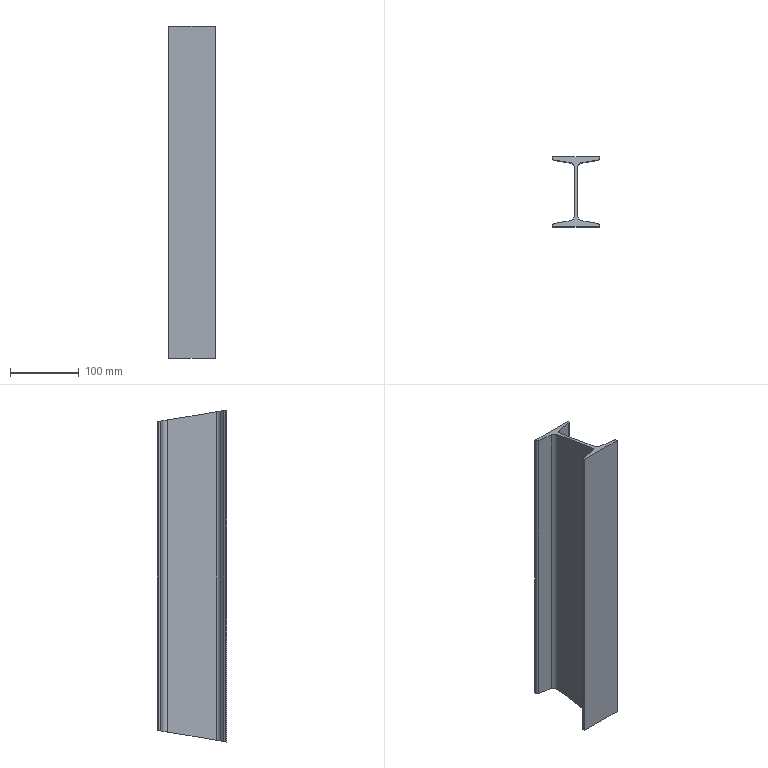Part | SolidWorks | features BaseBody 1 | 1 solid | 22 faces | box 67.6 x 101.6 x 482.765 mm | volume 647373 mm3 | plane 14 | cylinder 8 | commonest cylinder face diameters 5.6 x4 14.8 x4
STEP:
#1=CARTESIAN_POINT('',(-9.126,-3.883,0.));
#2=VERTEX_POINT('',#1);
#3=CARTESIAN_POINT('',(58.474,-3.883,0.));
#4=VERTEX_POINT('',#3);
#5=CARTESIAN_POINT('',(58.474,-3.883,0.));
#6=DIRECTION('',(1.,0.,0.));
#7=VECTOR('',#6,1000.);
#8=LINE('',#5,#7);
#9=EDGE_CURVE('',#2,#4,#8,.T.);
#10=ORIENTED_EDGE('',*,*,#9,.T.);
#11=CARTESIAN_POINT('',(58.474,-3.883,482.765));
#12=VERTEX_POINT('',#11);
#13=CARTESIAN_POINT('',(58.474,-3.883,0.));
#14=DIRECTION('',(0.,0.,1.));
#15=VECTOR('',#14,1000.);
#16=LINE('',#13,#15);
#17=EDGE_CURVE('',#4,#12,#16,.T.);
#18=ORIENTED_EDGE('',*,*,#17,.T.);
#19=CARTESIAN_POINT('',(-9.126,-3.883,482.765));
#20=VERTEX_POINT('',#19);
#21=CARTESIAN_POINT('',(58.474,-3.883,482.765));
#22=DIRECTION('',(-1.,0.,0.));
#23=VECTOR('',#22,1000.);
#24=LINE('',#21,#23);
#25=EDGE_CURVE('',#12,#20,#24,.T.);
#26=ORIENTED_EDGE('',*,*,#25,.T.);
#27=CARTESIAN_POINT('',(-9.126,-3.883,0.));
#28=DIRECTION('',(0.,0.,-1.));
#29=VECTOR('',#28,1000.);
#30=LINE('',#27,#29);
#31=EDGE_CURVE('',#20,#2,#30,.T.);
#32=ORIENTED_EDGE('',*,*,#31,.T.);
#33=EDGE_LOOP('',(#10,#18,#26,#32));
#34=FACE_OUTER_BOUND('',#33,.T.);
#35=CARTESIAN_POINT('',(58.474,-3.883,0.));
#36=DIRECTION('',(0.,-1.,0.));
#37=DIRECTION('',(0.,0.,-1.));
#38=AXIS2_PLACEMENT_3D('',#35,#36,#37);
#39=PLANE('',#38);
#40=ADVANCED_FACE('',(#34),#39,.T.);
#41=CARTESIAN_POINT('',(58.474,-1.913,482.435));
#42=VERTEX_POINT('',#41);
#43=CARTESIAN_POINT('',(58.474,-1.913,482.435));
#44=DIRECTION('',(0.,-0.9863,0.165));
#45=VECTOR('',#44,1000.);
#46=LINE('',#43,#45);
#47=EDGE_CURVE('',#42,#12,#46,.T.);
#48=ORIENTED_EDGE('',*,*,#47,.T.);
#49=ORIENTED_EDGE('',*,*,#17,.F.);
#50=CARTESIAN_POINT('',(58.474,-1.913,0.3297));
#51=VERTEX_POINT('',#50);
#52=CARTESIAN_POINT('',(58.474,-3.883,0.));
#53=DIRECTION('',(0.,0.9863,0.165));
#54=VECTOR('',#53,1000.);
#55=LINE('',#52,#54);
#56=EDGE_CURVE('',#4,#51,#55,.T.);
#57=ORIENTED_EDGE('',*,*,#56,.T.);
#58=CARTESIAN_POINT('',(58.474,-1.913,0.));
#59=DIRECTION('',(0.,0.,1.));
#60=VECTOR('',#59,1000.);
#61=LINE('',#58,#60);
#62=EDGE_CURVE('',#51,#42,#61,.T.);
#63=ORIENTED_EDGE('',*,*,#62,.T.);
#64=EDGE_LOOP('',(#48,#49,#57,#63));
#65=FACE_OUTER_BOUND('',#64,.T.);
#66=CARTESIAN_POINT('',(58.474,-1.913,0.));
#67=DIRECTION('',(1.,0.,0.));
#68=DIRECTION('',(0.,0.,-1.));
#69=AXIS2_PLACEMENT_3D('',#66,#67,#68);
#70=PLANE('',#69);
#71=ADVANCED_FACE('',(#65),#70,.T.);
#72=CARTESIAN_POINT('',(33.252,4.678,1.433));
#73=VERTEX_POINT('',#72);
#74=CARTESIAN_POINT('',(56.136,0.8486,0.7919));
#75=VERTEX_POINT('',#74);
#76=CARTESIAN_POINT('',(33.252,4.678,1.433));
#77=DIRECTION('',(0.9859,-0.165,-0.02761));
#78=VECTOR('',#77,1000.);
#79=LINE('',#76,#78);
#80=EDGE_CURVE('',#73,#75,#79,.T.);
#81=ORIENTED_EDGE('',*,*,#80,.T.);
#82=CARTESIAN_POINT('',(56.136,0.8486,0.7919));
#83=CARTESIAN_POINT('',(57.548,0.6122,0.7523));
#84=CARTESIAN_POINT('',(58.474,-0.4808,0.5694));
#85=CARTESIAN_POINT('',(58.474,-1.913,0.3297));
#86=(BOUNDED_CURVE()B_SPLINE_CURVE(3,(#82,#83,#84,#85),.UNSPECIFIED.,.F.,.F.)B_SPLINE_CURVE_WITH_KNOTS((4,4),(0.1658,1.571),.UNSPECIFIED.)CURVE()GEOMETRIC_REPRESENTATION_ITEM()RATIONAL_B_SPLINE_CURVE((1.,0.8422,0.8422,1.))REPRESENTATION_ITEM(''));
#87=EDGE_CURVE('',#75,#51,#86,.T.);
#88=ORIENTED_EDGE('',*,*,#87,.T.);
#89=ORIENTED_EDGE('',*,*,#56,.F.);
#90=ORIENTED_EDGE('',*,*,#9,.F.);
#91=CARTESIAN_POINT('',(-9.126,-1.913,0.3297));
#92=VERTEX_POINT('',#91);
#93=CARTESIAN_POINT('',(-9.126,46.917,8.501));
#94=DIRECTION('',(0.,0.9863,0.165));
#95=VECTOR('',#94,1000.);
#96=LINE('',#93,#95);
#97=EDGE_CURVE('',#2,#92,#96,.T.);
#98=ORIENTED_EDGE('',*,*,#97,.T.);
#99=CARTESIAN_POINT('',(-6.788,0.8486,0.7919));
#100=VERTEX_POINT('',#99);
#101=CARTESIAN_POINT('',(-9.126,-1.913,0.3297));
#102=CARTESIAN_POINT('',(-9.126,-0.4808,0.5694));
#103=CARTESIAN_POINT('',(-8.201,0.6122,0.7523));
#104=CARTESIAN_POINT('',(-6.788,0.8486,0.7919));
#105=(BOUNDED_CURVE()B_SPLINE_CURVE(3,(#101,#102,#103,#104),.UNSPECIFIED.,.F.,.T.)B_SPLINE_CURVE_WITH_KNOTS((4,4),(4.712,6.117),.UNSPECIFIED.)CURVE()GEOMETRIC_REPRESENTATION_ITEM()RATIONAL_B_SPLINE_CURVE((1.,0.8422,0.8422,1.))REPRESENTATION_ITEM(''));
#106=EDGE_CURVE('',#92,#100,#105,.T.);
#107=ORIENTED_EDGE('',*,*,#106,.T.);
#108=CARTESIAN_POINT('',(16.095,4.678,1.433));
#109=VERTEX_POINT('',#108);
#110=CARTESIAN_POINT('',(-6.788,0.8486,0.7919));
#111=DIRECTION('',(0.9859,0.165,0.02761));
#112=VECTOR('',#111,1000.);
#113=LINE('',#110,#112);
#114=EDGE_CURVE('',#100,#109,#113,.T.);
#115=ORIENTED_EDGE('',*,*,#114,.T.);
#116=CARTESIAN_POINT('',(22.274,11.977,2.654));
#117=VERTEX_POINT('',#116);
#118=CARTESIAN_POINT('',(16.095,4.678,1.433));
#119=CARTESIAN_POINT('',(19.828,5.303,1.537));
#120=CARTESIAN_POINT('',(22.274,8.192,2.021));
#121=CARTESIAN_POINT('',(22.274,11.977,2.654));
#122=(BOUNDED_CURVE()B_SPLINE_CURVE(3,(#118,#119,#120,#121),.UNSPECIFIED.,.F.,.F.)B_SPLINE_CURVE_WITH_KNOTS((4,4),(3.307,4.712),.UNSPECIFIED.)CURVE()GEOMETRIC_REPRESENTATION_ITEM()RATIONAL_B_SPLINE_CURVE((1.,0.8422,0.8422,1.))REPRESENTATION_ITEM(''));
#123=EDGE_CURVE('',#109,#117,#122,.T.);
#124=ORIENTED_EDGE('',*,*,#123,.T.);
#125=CARTESIAN_POINT('',(22.274,81.857,14.348));
#126=VERTEX_POINT('',#125);
#127=CARTESIAN_POINT('',(22.274,46.917,8.501));
#128=DIRECTION('',(0.,0.9863,0.165));
#129=VECTOR('',#128,1000.);
#130=LINE('',#127,#129);
#131=EDGE_CURVE('',#117,#126,#130,.T.);
#132=ORIENTED_EDGE('',*,*,#131,.T.);
#133=CARTESIAN_POINT('',(16.095,89.155,15.569));
#134=VERTEX_POINT('',#133);
#135=CARTESIAN_POINT('',(22.274,81.857,14.348));
#136=CARTESIAN_POINT('',(22.274,85.642,14.981));
#137=CARTESIAN_POINT('',(19.828,88.53,15.465));
#138=CARTESIAN_POINT('',(16.095,89.155,15.569));
#139=(BOUNDED_CURVE()B_SPLINE_CURVE(3,(#135,#136,#137,#138),.UNSPECIFIED.,.F.,.F.)B_SPLINE_CURVE_WITH_KNOTS((4,4),(4.712,6.117),.UNSPECIFIED.)CURVE()GEOMETRIC_REPRESENTATION_ITEM()RATIONAL_B_SPLINE_CURVE((1.,0.8422,0.8422,1.))REPRESENTATION_ITEM(''));
#140=EDGE_CURVE('',#126,#134,#139,.T.);
#141=ORIENTED_EDGE('',*,*,#140,.T.);
#142=CARTESIAN_POINT('',(-6.788,92.984,16.21));
#143=VERTEX_POINT('',#142);
#144=CARTESIAN_POINT('',(16.095,89.155,15.569));
#145=DIRECTION('',(-0.9859,0.165,0.02761));
#146=VECTOR('',#145,1000.);
#147=LINE('',#144,#146);
#148=EDGE_CURVE('',#134,#143,#147,.T.);
#149=ORIENTED_EDGE('',*,*,#148,.T.);
#150=CARTESIAN_POINT('',(-9.126,95.746,16.672));
#151=VERTEX_POINT('',#150);
#152=CARTESIAN_POINT('',(-6.788,92.984,16.21));
#153=CARTESIAN_POINT('',(-8.201,93.221,16.25));
#154=CARTESIAN_POINT('',(-9.126,94.314,16.433));
#155=CARTESIAN_POINT('',(-9.126,95.746,16.672));
#156=(BOUNDED_CURVE()B_SPLINE_CURVE(3,(#152,#153,#154,#155),.UNSPECIFIED.,.F.,.F.)B_SPLINE_CURVE_WITH_KNOTS((4,4),(3.307,4.712),.UNSPECIFIED.)CURVE()GEOMETRIC_REPRESENTATION_ITEM()RATIONAL_B_SPLINE_CURVE((1.,0.8422,0.8422,1.))REPRESENTATION_ITEM(''));
#157=EDGE_CURVE('',#143,#151,#156,.T.);
#158=ORIENTED_EDGE('',*,*,#157,.T.);
#159=CARTESIAN_POINT('',(-9.126,97.717,17.002));
#160=VERTEX_POINT('',#159);
#161=CARTESIAN_POINT('',(-9.126,46.917,8.501));
#162=DIRECTION('',(0.,0.9863,0.165));
#163=VECTOR('',#162,1000.);
#164=LINE('',#161,#163);
#165=EDGE_CURVE('',#151,#160,#164,.T.);
#166=ORIENTED_EDGE('',*,*,#165,.T.);
#167=CARTESIAN_POINT('',(58.474,97.717,17.002));
#168=VERTEX_POINT('',#167);
#169=CARTESIAN_POINT('',(7.774,97.717,17.002));
#170=DIRECTION('',(1.,0.,0.));
#171=VECTOR('',#170,1000.);
#172=LINE('',#169,#171);
#173=EDGE_CURVE('',#160,#168,#172,.T.);
#174=ORIENTED_EDGE('',*,*,#173,.T.);
#175=CARTESIAN_POINT('',(58.474,95.746,16.672));
#176=VERTEX_POINT('',#175);
#177=CARTESIAN_POINT('',(58.474,46.917,8.501));
#178=DIRECTION('',(0.,-0.9863,-0.165));
#179=VECTOR('',#178,1000.);
#180=LINE('',#177,#179);
#181=EDGE_CURVE('',#168,#176,#180,.T.);
#182=ORIENTED_EDGE('',*,*,#181,.T.);
#183=CARTESIAN_POINT('',(56.136,92.984,16.21));
#184=VERTEX_POINT('',#183);
#185=CARTESIAN_POINT('',(58.474,95.746,16.672));
#186=CARTESIAN_POINT('',(58.474,94.314,16.433));
#187=CARTESIAN_POINT('',(57.548,93.221,16.25));
#188=CARTESIAN_POINT('',(56.136,92.984,16.21));
#189=(BOUNDED_CURVE()B_SPLINE_CURVE(3,(#185,#186,#187,#188),.UNSPECIFIED.,.F.,.F.)B_SPLINE_CURVE_WITH_KNOTS((4,4),(1.571,2.976),.UNSPECIFIED.)CURVE()GEOMETRIC_REPRESENTATION_ITEM()RATIONAL_B_SPLINE_CURVE((1.,0.8422,0.8422,1.))REPRESENTATION_ITEM(''));
#190=EDGE_CURVE('',#176,#184,#189,.T.);
#191=ORIENTED_EDGE('',*,*,#190,.T.);
#192=CARTESIAN_POINT('',(33.252,89.155,15.569));
#193=VERTEX_POINT('',#192);
#194=CARTESIAN_POINT('',(56.136,92.984,16.21));
#195=DIRECTION('',(-0.9859,-0.165,-0.02761));
#196=VECTOR('',#195,1000.);
#197=LINE('',#194,#196);
#198=EDGE_CURVE('',#184,#193,#197,.T.);
#199=ORIENTED_EDGE('',*,*,#198,.T.);
#200=CARTESIAN_POINT('',(27.074,81.857,14.348));
#201=VERTEX_POINT('',#200);
#202=CARTESIAN_POINT('',(33.252,89.155,15.569));
#203=CARTESIAN_POINT('',(29.519,88.53,15.465));
#204=CARTESIAN_POINT('',(27.074,85.642,14.981));
#205=CARTESIAN_POINT('',(27.074,81.857,14.348));
#206=(BOUNDED_CURVE()B_SPLINE_CURVE(3,(#202,#203,#204,#205),.UNSPECIFIED.,.F.,.F.)B_SPLINE_CURVE_WITH_KNOTS((4,4),(0.1658,1.571),.UNSPECIFIED.)CURVE()GEOMETRIC_REPRESENTATION_ITEM()RATIONAL_B_SPLINE_CURVE((1.,0.8422,0.8422,1.))REPRESENTATION_ITEM(''));
#207=EDGE_CURVE('',#193,#201,#206,.T.);
#208=ORIENTED_EDGE('',*,*,#207,.T.);
#209=CARTESIAN_POINT('',(27.074,11.977,2.654));
#210=VERTEX_POINT('',#209);
#211=CARTESIAN_POINT('',(27.074,46.917,8.501));
#212=DIRECTION('',(0.,-0.9863,-0.165));
#213=VECTOR('',#212,1000.);
#214=LINE('',#211,#213);
#215=EDGE_CURVE('',#201,#210,#214,.T.);
#216=ORIENTED_EDGE('',*,*,#215,.T.);
#217=CARTESIAN_POINT('',(27.074,11.977,2.654));
#218=CARTESIAN_POINT('',(27.074,8.192,2.021));
#219=CARTESIAN_POINT('',(29.519,5.303,1.537));
#220=CARTESIAN_POINT('',(33.252,4.678,1.433));
#221=(BOUNDED_CURVE()B_SPLINE_CURVE(3,(#217,#218,#219,#220),.UNSPECIFIED.,.F.,.F.)B_SPLINE_CURVE_WITH_KNOTS((4,4),(1.571,2.976),.UNSPECIFIED.)CURVE()GEOMETRIC_REPRESENTATION_ITEM()RATIONAL_B_SPLINE_CURVE((1.,0.8422,0.8422,1.))REPRESENTATION_ITEM(''));
#222=EDGE_CURVE('',#210,#73,#221,.T.);
#223=ORIENTED_EDGE('',*,*,#222,.T.);
#224=EDGE_LOOP('',(#81,#88,#89,#90,#98,#107,#115,#124,#132,#141,#149,#158,#166,#174,#182,#191,#199,#208,#216,#223));
#225=FACE_OUTER_BOUND('',#224,.T.);
#226=CARTESIAN_POINT('',(7.774,46.917,8.501));
#227=DIRECTION('',(0.,0.165,-0.9863));
#228=DIRECTION('',(0.,0.9863,0.165));
#229=AXIS2_PLACEMENT_3D('',#226,#227,#228);
#230=PLANE('',#229);
#231=ADVANCED_FACE('',(#225),#230,.T.);
#232=CARTESIAN_POINT('',(-9.126,-1.913,482.435));
#233=VERTEX_POINT('',#232);
#234=CARTESIAN_POINT('',(-9.126,-3.883,482.765));
#235=DIRECTION('',(0.,0.9863,-0.165));
#236=VECTOR('',#235,1000.);
#237=LINE('',#234,#236);
#238=EDGE_CURVE('',#20,#233,#237,.T.);
#239=ORIENTED_EDGE('',*,*,#238,.T.);
#240=CARTESIAN_POINT('',(-9.126,-1.913,0.));
#241=DIRECTION('',(0.,0.,-1.));
#242=VECTOR('',#241,1000.);
#243=LINE('',#240,#242);
#244=EDGE_CURVE('',#233,#92,#243,.T.);
#245=ORIENTED_EDGE('',*,*,#244,.T.);
#246=ORIENTED_EDGE('',*,*,#97,.F.);
#247=ORIENTED_EDGE('',*,*,#31,.F.);
#248=EDGE_LOOP('',(#239,#245,#246,#247));
#249=FACE_OUTER_BOUND('',#248,.T.);
#250=CARTESIAN_POINT('',(-9.126,-3.883,0.));
#251=DIRECTION('',(-1.,0.,0.));
#252=DIRECTION('',(0.,0.,1.));
#253=AXIS2_PLACEMENT_3D('',#250,#251,#252);
#254=PLANE('',#253);
#255=ADVANCED_FACE('',(#249),#254,.T.);
#256=CARTESIAN_POINT('',(33.252,89.155,467.196));
#257=VERTEX_POINT('',#256);
#258=CARTESIAN_POINT('',(56.136,92.984,466.555));
#259=VERTEX_POINT('',#258);
#260=CARTESIAN_POINT('',(33.252,89.155,467.196));
#261=DIRECTION('',(0.9859,0.165,-0.02761));
#262=VECTOR('',#261,1000.);
#263=LINE('',#260,#262);
#264=EDGE_CURVE('',#257,#259,#263,.T.);
#265=ORIENTED_EDGE('',*,*,#264,.T.);
#266=CARTESIAN_POINT('',(58.474,95.746,466.093));
#267=VERTEX_POINT('',#266);
#268=CARTESIAN_POINT('',(56.136,92.984,466.555));
#269=CARTESIAN_POINT('',(57.548,93.221,466.515));
#270=CARTESIAN_POINT('',(58.474,94.314,466.332));
#271=CARTESIAN_POINT('',(58.474,95.746,466.093));
#272=(BOUNDED_CURVE()B_SPLINE_CURVE(3,(#268,#269,#270,#271),.UNSPECIFIED.,.F.,.F.)B_SPLINE_CURVE_WITH_KNOTS((4,4),(0.1658,1.571),.UNSPECIFIED.)CURVE()GEOMETRIC_REPRESENTATION_ITEM()RATIONAL_B_SPLINE_CURVE((1.,0.8422,0.8422,1.))REPRESENTATION_ITEM(''));
#273=EDGE_CURVE('',#259,#267,#272,.T.);
#274=ORIENTED_EDGE('',*,*,#273,.T.);
#275=CARTESIAN_POINT('',(58.474,97.717,465.763));
#276=VERTEX_POINT('',#275);
#277=CARTESIAN_POINT('',(58.474,46.917,474.264));
#278=DIRECTION('',(0.,0.9863,-0.165));
#279=VECTOR('',#278,1000.);
#280=LINE('',#277,#279);
#281=EDGE_CURVE('',#267,#276,#280,.T.);
#282=ORIENTED_EDGE('',*,*,#281,.T.);
#283=CARTESIAN_POINT('',(-9.126,97.717,465.763));
#284=VERTEX_POINT('',#283);
#285=CARTESIAN_POINT('',(7.774,97.717,465.763));
#286=DIRECTION('',(-1.,0.,0.));
#287=VECTOR('',#286,1000.);
#288=LINE('',#285,#287);
#289=EDGE_CURVE('',#276,#284,#288,.T.);
#290=ORIENTED_EDGE('',*,*,#289,.T.);
#291=CARTESIAN_POINT('',(-9.126,95.746,466.093));
#292=VERTEX_POINT('',#291);
#293=CARTESIAN_POINT('',(-9.126,46.917,474.264));
#294=DIRECTION('',(0.,-0.9863,0.165));
#295=VECTOR('',#294,1000.);
#296=LINE('',#293,#295);
#297=EDGE_CURVE('',#284,#292,#296,.T.);
#298=ORIENTED_EDGE('',*,*,#297,.T.);
#299=CARTESIAN_POINT('',(-6.788,92.984,466.555));
#300=VERTEX_POINT('',#299);
#301=CARTESIAN_POINT('',(-9.126,95.746,466.093));
#302=CARTESIAN_POINT('',(-9.126,94.314,466.332));
#303=CARTESIAN_POINT('',(-8.201,93.221,466.515));
#304=CARTESIAN_POINT('',(-6.788,92.984,466.555));
#305=(BOUNDED_CURVE()B_SPLINE_CURVE(3,(#301,#302,#303,#304),.UNSPECIFIED.,.F.,.F.)B_SPLINE_CURVE_WITH_KNOTS((4,4),(4.712,6.117),.UNSPECIFIED.)CURVE()GEOMETRIC_REPRESENTATION_ITEM()RATIONAL_B_SPLINE_CURVE((1.,0.8422,0.8422,1.))REPRESENTATION_ITEM(''));
#306=EDGE_CURVE('',#292,#300,#305,.T.);
#307=ORIENTED_EDGE('',*,*,#306,.T.);
#308=CARTESIAN_POINT('',(16.095,89.155,467.196));
#309=VERTEX_POINT('',#308);
#310=CARTESIAN_POINT('',(-6.788,92.984,466.555));
#311=DIRECTION('',(0.9859,-0.165,0.02761));
#312=VECTOR('',#311,1000.);
#313=LINE('',#310,#312);
#314=EDGE_CURVE('',#300,#309,#313,.T.);
#315=ORIENTED_EDGE('',*,*,#314,.T.);
#316=CARTESIAN_POINT('',(22.274,81.857,468.417));
#317=VERTEX_POINT('',#316);
#318=CARTESIAN_POINT('',(16.095,89.155,467.196));
#319=CARTESIAN_POINT('',(19.828,88.53,467.3));
#320=CARTESIAN_POINT('',(22.274,85.642,467.784));
#321=CARTESIAN_POINT('',(22.274,81.857,468.417));
#322=(BOUNDED_CURVE()B_SPLINE_CURVE(3,(#318,#319,#320,#321),.UNSPECIFIED.,.F.,.F.)B_SPLINE_CURVE_WITH_KNOTS((4,4),(3.307,4.712),.UNSPECIFIED.)CURVE()GEOMETRIC_REPRESENTATION_ITEM()RATIONAL_B_SPLINE_CURVE((1.,0.8422,0.8422,1.))REPRESENTATION_ITEM(''));
#323=EDGE_CURVE('',#309,#317,#322,.T.);
#324=ORIENTED_EDGE('',*,*,#323,.T.);
#325=CARTESIAN_POINT('',(22.274,11.977,480.111));
#326=VERTEX_POINT('',#325);
#327=CARTESIAN_POINT('',(22.274,46.917,474.264));
#328=DIRECTION('',(0.,-0.9863,0.165));
#329=VECTOR('',#328,1000.);
#330=LINE('',#327,#329);
#331=EDGE_CURVE('',#317,#326,#330,.T.);
#332=ORIENTED_EDGE('',*,*,#331,.T.);
#333=CARTESIAN_POINT('',(16.095,4.678,481.332));
#334=VERTEX_POINT('',#333);
#335=CARTESIAN_POINT('',(22.274,11.977,480.111));
#336=CARTESIAN_POINT('',(22.274,8.192,480.744));
#337=CARTESIAN_POINT('',(19.828,5.303,481.228));
#338=CARTESIAN_POINT('',(16.095,4.678,481.332));
#339=(BOUNDED_CURVE()B_SPLINE_CURVE(3,(#335,#336,#337,#338),.UNSPECIFIED.,.F.,.F.)B_SPLINE_CURVE_WITH_KNOTS((4,4),(4.712,6.117),.UNSPECIFIED.)CURVE()GEOMETRIC_REPRESENTATION_ITEM()RATIONAL_B_SPLINE_CURVE((1.,0.8422,0.8422,1.))REPRESENTATION_ITEM(''));
#340=EDGE_CURVE('',#326,#334,#339,.T.);
#341=ORIENTED_EDGE('',*,*,#340,.T.);
#342=CARTESIAN_POINT('',(-6.788,0.8486,481.973));
#343=VERTEX_POINT('',#342);
#344=CARTESIAN_POINT('',(16.095,4.678,481.332));
#345=DIRECTION('',(-0.9859,-0.165,0.02761));
#346=VECTOR('',#345,1000.);
#347=LINE('',#344,#346);
#348=EDGE_CURVE('',#334,#343,#347,.T.);
#349=ORIENTED_EDGE('',*,*,#348,.T.);
#350=CARTESIAN_POINT('',(-6.788,0.8486,481.973));
#351=CARTESIAN_POINT('',(-8.201,0.6122,482.013));
#352=CARTESIAN_POINT('',(-9.126,-0.4808,482.196));
#353=CARTESIAN_POINT('',(-9.126,-1.913,482.435));
#354=(BOUNDED_CURVE()B_SPLINE_CURVE(3,(#350,#351,#352,#353),.UNSPECIFIED.,.F.,.F.)B_SPLINE_CURVE_WITH_KNOTS((4,4),(3.307,4.712),.UNSPECIFIED.)CURVE()GEOMETRIC_REPRESENTATION_ITEM()RATIONAL_B_SPLINE_CURVE((1.,0.8422,0.8422,1.))REPRESENTATION_ITEM(''));
#355=EDGE_CURVE('',#343,#233,#354,.T.);
#356=ORIENTED_EDGE('',*,*,#355,.T.);
#357=ORIENTED_EDGE('',*,*,#238,.F.);
#358=ORIENTED_EDGE('',*,*,#25,.F.);
#359=ORIENTED_EDGE('',*,*,#47,.F.);
#360=CARTESIAN_POINT('',(56.136,0.8486,481.973));
#361=VERTEX_POINT('',#360);
#362=CARTESIAN_POINT('',(58.474,-1.913,482.435));
#363=CARTESIAN_POINT('',(58.474,-0.4808,482.196));
#364=CARTESIAN_POINT('',(57.548,0.6122,482.013));
#365=CARTESIAN_POINT('',(56.136,0.8486,481.973));
#366=(BOUNDED_CURVE()B_SPLINE_CURVE(3,(#362,#363,#364,#365),.UNSPECIFIED.,.F.,.F.)B_SPLINE_CURVE_WITH_KNOTS((4,4),(1.571,2.976),.UNSPECIFIED.)CURVE()GEOMETRIC_REPRESENTATION_ITEM()RATIONAL_B_SPLINE_CURVE((1.,0.8422,0.8422,1.))REPRESENTATION_ITEM(''));
#367=EDGE_CURVE('',#42,#361,#366,.T.);
#368=ORIENTED_EDGE('',*,*,#367,.T.);
#369=CARTESIAN_POINT('',(33.252,4.678,481.332));
#370=VERTEX_POINT('',#369);
#371=CARTESIAN_POINT('',(56.136,0.8486,481.973));
#372=DIRECTION('',(-0.9859,0.165,-0.02761));
#373=VECTOR('',#372,1000.);
#374=LINE('',#371,#373);
#375=EDGE_CURVE('',#361,#370,#374,.T.);
#376=ORIENTED_EDGE('',*,*,#375,.T.);
#377=CARTESIAN_POINT('',(27.074,11.977,480.111));
#378=VERTEX_POINT('',#377);
#379=CARTESIAN_POINT('',(33.252,4.678,481.332));
#380=CARTESIAN_POINT('',(29.519,5.303,481.228));
#381=CARTESIAN_POINT('',(27.074,8.192,480.744));
#382=CARTESIAN_POINT('',(27.074,11.977,480.111));
#383=(BOUNDED_CURVE()B_SPLINE_CURVE(3,(#379,#380,#381,#382),.UNSPECIFIED.,.F.,.T.)B_SPLINE_CURVE_WITH_KNOTS((4,4),(0.1658,1.571),.UNSPECIFIED.)CURVE()GEOMETRIC_REPRESENTATION_ITEM()RATIONAL_B_SPLINE_CURVE((1.,0.8422,0.8422,1.))REPRESENTATION_ITEM(''));
#384=EDGE_CURVE('',#370,#378,#383,.T.);
#385=ORIENTED_EDGE('',*,*,#384,.T.);
#386=CARTESIAN_POINT('',(27.074,81.857,468.417));
#387=VERTEX_POINT('',#386);
#388=CARTESIAN_POINT('',(27.074,46.917,474.264));
#389=DIRECTION('',(0.,0.9863,-0.165));
#390=VECTOR('',#389,1000.);
#391=LINE('',#388,#390);
#392=EDGE_CURVE('',#378,#387,#391,.T.);
#393=ORIENTED_EDGE('',*,*,#392,.T.);
#394=CARTESIAN_POINT('',(27.074,81.857,468.417));
#395=CARTESIAN_POINT('',(27.074,85.642,467.784));
#396=CARTESIAN_POINT('',(29.519,88.53,467.3));
#397=CARTESIAN_POINT('',(33.252,89.155,467.196));
#398=(BOUNDED_CURVE()B_SPLINE_CURVE(3,(#394,#395,#396,#397),.UNSPECIFIED.,.F.,.F.)B_SPLINE_CURVE_WITH_KNOTS((4,4),(1.571,2.976),.UNSPECIFIED.)CURVE()GEOMETRIC_REPRESENTATION_ITEM()RATIONAL_B_SPLINE_CURVE((1.,0.8422,0.8422,1.))REPRESENTATION_ITEM(''));
#399=EDGE_CURVE('',#387,#257,#398,.T.);
#400=ORIENTED_EDGE('',*,*,#399,.T.);
#401=EDGE_LOOP('',(#265,#274,#282,#290,#298,#307,#315,#324,#332,#341,#349,#356,#357,#358,#359,#368,#376,#385,#393,#400));
#402=FACE_OUTER_BOUND('',#401,.T.);
#403=CARTESIAN_POINT('',(7.774,46.917,474.264));
#404=DIRECTION('',(0.,0.165,0.9863));
#405=DIRECTION('',(0.,-0.9863,0.165));
#406=AXIS2_PLACEMENT_3D('',#403,#404,#405);
#407=PLANE('',#406);
#408=ADVANCED_FACE('',(#402),#407,.T.);
#409=ORIENTED_EDGE('',*,*,#367,.F.);
#410=ORIENTED_EDGE('',*,*,#62,.F.);
#411=ORIENTED_EDGE('',*,*,#87,.F.);
#412=CARTESIAN_POINT('',(56.136,0.8486,0.));
#413=DIRECTION('',(0.,0.,1.));
#414=VECTOR('',#413,1000.);
#415=LINE('',#412,#414);
#416=EDGE_CURVE('',#75,#361,#415,.T.);
#417=ORIENTED_EDGE('',*,*,#416,.T.);
#418=EDGE_LOOP('',(#409,#410,#411,#417));
#419=FACE_OUTER_BOUND('',#418,.T.);
#420=CARTESIAN_POINT('',(55.674,-1.913,0.));
#421=DIRECTION('',(0.,0.,1.));
#422=DIRECTION('',(1.,0.,0.));
#423=AXIS2_PLACEMENT_3D('',#420,#421,#422);
#424=CYLINDRICAL_SURFACE('',#423,2.8);
#425=ADVANCED_FACE('',(#419),#424,.T.);
#426=ORIENTED_EDGE('',*,*,#375,.F.);
#427=ORIENTED_EDGE('',*,*,#416,.F.);
#428=ORIENTED_EDGE('',*,*,#80,.F.);
#429=CARTESIAN_POINT('',(33.252,4.678,0.));
#430=DIRECTION('',(0.,0.,1.));
#431=VECTOR('',#430,1000.);
#432=LINE('',#429,#431);
#433=EDGE_CURVE('',#73,#370,#432,.T.);
#434=ORIENTED_EDGE('',*,*,#433,.T.);
#435=EDGE_LOOP('',(#426,#427,#428,#434));
#436=FACE_OUTER_BOUND('',#435,.T.);
#437=CARTESIAN_POINT('',(33.252,4.678,0.));
#438=DIRECTION('',(0.165,0.9863,0.));
#439=DIRECTION('',(-0.9863,0.165,0.));
#440=AXIS2_PLACEMENT_3D('',#437,#438,#439);
#441=PLANE('',#440);
#442=ADVANCED_FACE('',(#436),#441,.T.);
#443=CARTESIAN_POINT('',(27.074,11.977,0.));
#444=DIRECTION('',(0.,0.,-1.));
#445=VECTOR('',#444,1000.);
#446=LINE('',#443,#445);
#447=EDGE_CURVE('',#378,#210,#446,.T.);
#448=ORIENTED_EDGE('',*,*,#447,.F.);
#449=ORIENTED_EDGE('',*,*,#384,.F.);
#450=ORIENTED_EDGE('',*,*,#433,.F.);
#451=ORIENTED_EDGE('',*,*,#222,.F.);
#452=EDGE_LOOP('',(#448,#449,#450,#451));
#453=FACE_OUTER_BOUND('',#452,.T.);
#454=CARTESIAN_POINT('',(34.474,11.977,0.));
#455=DIRECTION('',(0.,0.,1.));
#456=DIRECTION('',(1.,0.,0.));
#457=AXIS2_PLACEMENT_3D('',#454,#455,#456);
#458=CYLINDRICAL_SURFACE('',#457,7.4);
#459=ADVANCED_FACE('',(#453),#458,.F.);
#460=ORIENTED_EDGE('',*,*,#392,.F.);
#461=ORIENTED_EDGE('',*,*,#447,.T.);
#462=ORIENTED_EDGE('',*,*,#215,.F.);
#463=CARTESIAN_POINT('',(27.074,81.857,0.));
#464=DIRECTION('',(0.,0.,1.));
#465=VECTOR('',#464,1000.);
#466=LINE('',#463,#465);
#467=EDGE_CURVE('',#201,#387,#466,.T.);
#468=ORIENTED_EDGE('',*,*,#467,.T.);
#469=EDGE_LOOP('',(#460,#461,#462,#468));
#470=FACE_OUTER_BOUND('',#469,.T.);
#471=CARTESIAN_POINT('',(27.074,81.857,0.));
#472=DIRECTION('',(1.,0.,0.));
#473=DIRECTION('',(0.,0.,-1.));
#474=AXIS2_PLACEMENT_3D('',#471,#472,#473);
#475=PLANE('',#474);
#476=ADVANCED_FACE('',(#470),#475,.T.);
#477=CARTESIAN_POINT('',(33.252,89.155,0.));
#478=DIRECTION('',(0.,0.,-1.));
#479=VECTOR('',#478,1000.);
#480=LINE('',#477,#479);
#481=EDGE_CURVE('',#257,#193,#480,.T.);
#482=ORIENTED_EDGE('',*,*,#481,.F.);
#483=ORIENTED_EDGE('',*,*,#399,.F.);
#484=ORIENTED_EDGE('',*,*,#467,.F.);
#485=ORIENTED_EDGE('',*,*,#207,.F.);
#486=EDGE_LOOP('',(#482,#483,#484,#485));
#487=FACE_OUTER_BOUND('',#486,.T.);
#488=CARTESIAN_POINT('',(34.474,81.857,0.));
#489=DIRECTION('',(0.,0.,1.));
#490=DIRECTION('',(1.,0.,0.));
#491=AXIS2_PLACEMENT_3D('',#488,#489,#490);
#492=CYLINDRICAL_SURFACE('',#491,7.4);
#493=ADVANCED_FACE('',(#487),#492,.F.);
#494=ORIENTED_EDGE('',*,*,#264,.F.);
#495=ORIENTED_EDGE('',*,*,#481,.T.);
#496=ORIENTED_EDGE('',*,*,#198,.F.);
#497=CARTESIAN_POINT('',(56.136,92.984,0.));
#498=DIRECTION('',(0.,0.,1.));
#499=VECTOR('',#498,1000.);
#500=LINE('',#497,#499);
#501=EDGE_CURVE('',#184,#259,#500,.T.);
#502=ORIENTED_EDGE('',*,*,#501,.T.);
#503=EDGE_LOOP('',(#494,#495,#496,#502));
#504=FACE_OUTER_BOUND('',#503,.T.);
#505=CARTESIAN_POINT('',(56.136,92.984,0.));
#506=DIRECTION('',(0.165,-0.9863,0.));
#507=DIRECTION('',(0.9863,0.165,0.));
#508=AXIS2_PLACEMENT_3D('',#505,#506,#507);
#509=PLANE('',#508);
#510=ADVANCED_FACE('',(#504),#509,.T.);
#511=ORIENTED_EDGE('',*,*,#273,.F.);
#512=ORIENTED_EDGE('',*,*,#501,.F.);
#513=ORIENTED_EDGE('',*,*,#190,.F.);
#514=CARTESIAN_POINT('',(58.474,95.746,0.));
#515=DIRECTION('',(0.,0.,1.));
#516=VECTOR('',#515,1000.);
#517=LINE('',#514,#516);
#518=EDGE_CURVE('',#176,#267,#517,.T.);
#519=ORIENTED_EDGE('',*,*,#518,.T.);
#520=EDGE_LOOP('',(#511,#512,#513,#519));
#521=FACE_OUTER_BOUND('',#520,.T.);
#522=CARTESIAN_POINT('',(55.674,95.746,0.));
#523=DIRECTION('',(0.,0.,1.));
#524=DIRECTION('',(1.,0.,0.));
#525=AXIS2_PLACEMENT_3D('',#522,#523,#524);
#526=CYLINDRICAL_SURFACE('',#525,2.8);
#527=ADVANCED_FACE('',(#521),#526,.T.);
#528=ORIENTED_EDGE('',*,*,#281,.F.);
#529=ORIENTED_EDGE('',*,*,#518,.F.);
#530=ORIENTED_EDGE('',*,*,#181,.F.);
#531=CARTESIAN_POINT('',(58.474,97.717,0.));
#532=DIRECTION('',(0.,0.,1.));
#533=VECTOR('',#532,1000.);
#534=LINE('',#531,#533);
#535=EDGE_CURVE('',#168,#276,#534,.T.);
#536=ORIENTED_EDGE('',*,*,#535,.T.);
#537=EDGE_LOOP('',(#528,#529,#530,#536));
#538=FACE_OUTER_BOUND('',#537,.T.);
#539=CARTESIAN_POINT('',(58.474,97.717,0.));
#540=DIRECTION('',(1.,0.,0.));
#541=DIRECTION('',(0.,0.,-1.));
#542=AXIS2_PLACEMENT_3D('',#539,#540,#541);
#543=PLANE('',#542);
#544=ADVANCED_FACE('',(#538),#543,.T.);
#545=ORIENTED_EDGE('',*,*,#289,.F.);
#546=ORIENTED_EDGE('',*,*,#535,.F.);
#547=ORIENTED_EDGE('',*,*,#173,.F.);
#548=CARTESIAN_POINT('',(-9.126,97.717,0.));
#549=DIRECTION('',(0.,0.,1.));
#550=VECTOR('',#549,1000.);
#551=LINE('',#548,#550);
#552=EDGE_CURVE('',#160,#284,#551,.T.);
#553=ORIENTED_EDGE('',*,*,#552,.T.);
#554=EDGE_LOOP('',(#545,#546,#547,#553));
#555=FACE_OUTER_BOUND('',#554,.T.);
#556=CARTESIAN_POINT('',(-9.126,97.717,0.));
#557=DIRECTION('',(0.,1.,0.));
#558=DIRECTION('',(0.,0.,1.));
#559=AXIS2_PLACEMENT_3D('',#556,#557,#558);
#560=PLANE('',#559);
#561=ADVANCED_FACE('',(#555),#560,.T.);
#562=ORIENTED_EDGE('',*,*,#297,.F.);
#563=ORIENTED_EDGE('',*,*,#552,.F.);
#564=ORIENTED_EDGE('',*,*,#165,.F.);
#565=CARTESIAN_POINT('',(-9.126,95.746,0.));
#566=DIRECTION('',(0.,0.,1.));
#567=VECTOR('',#566,1000.);
#568=LINE('',#565,#567);
#569=EDGE_CURVE('',#151,#292,#568,.T.);
#570=ORIENTED_EDGE('',*,*,#569,.T.);
#571=EDGE_LOOP('',(#562,#563,#564,#570));
#572=FACE_OUTER_BOUND('',#571,.T.);
#573=CARTESIAN_POINT('',(-9.126,95.746,0.));
#574=DIRECTION('',(-1.,0.,0.));
#575=DIRECTION('',(0.,0.,1.));
#576=AXIS2_PLACEMENT_3D('',#573,#574,#575);
#577=PLANE('',#576);
#578=ADVANCED_FACE('',(#572),#577,.T.);
#579=ORIENTED_EDGE('',*,*,#306,.F.);
#580=ORIENTED_EDGE('',*,*,#569,.F.);
#581=ORIENTED_EDGE('',*,*,#157,.F.);
#582=CARTESIAN_POINT('',(-6.788,92.984,0.));
#583=DIRECTION('',(0.,0.,1.));
#584=VECTOR('',#583,1000.);
#585=LINE('',#582,#584);
#586=EDGE_CURVE('',#143,#300,#585,.T.);
#587=ORIENTED_EDGE('',*,*,#586,.T.);
#588=EDGE_LOOP('',(#579,#580,#581,#587));
#589=FACE_OUTER_BOUND('',#588,.T.);
#590=CARTESIAN_POINT('',(-6.326,95.746,0.));
#591=DIRECTION('',(0.,0.,1.));
#592=DIRECTION('',(1.,0.,0.));
#593=AXIS2_PLACEMENT_3D('',#590,#591,#592);
#594=CYLINDRICAL_SURFACE('',#593,2.8);
#595=ADVANCED_FACE('',(#589),#594,.T.);
#596=ORIENTED_EDGE('',*,*,#314,.F.);
#597=ORIENTED_EDGE('',*,*,#586,.F.);
#598=ORIENTED_EDGE('',*,*,#148,.F.);
#599=CARTESIAN_POINT('',(16.095,89.155,0.));
#600=DIRECTION('',(0.,0.,1.));
#601=VECTOR('',#600,1000.);
#602=LINE('',#599,#601);
#603=EDGE_CURVE('',#134,#309,#602,.T.);
#604=ORIENTED_EDGE('',*,*,#603,.T.);
#605=EDGE_LOOP('',(#596,#597,#598,#604));
#606=FACE_OUTER_BOUND('',#605,.T.);
#607=CARTESIAN_POINT('',(16.095,89.155,0.));
#608=DIRECTION('',(-0.165,-0.9863,0.));
#609=DIRECTION('',(0.9863,-0.165,0.));
#610=AXIS2_PLACEMENT_3D('',#607,#608,#609);
#611=PLANE('',#610);
#612=ADVANCED_FACE('',(#606),#611,.T.);
#613=CARTESIAN_POINT('',(22.274,81.857,0.));
#614=DIRECTION('',(0.,0.,-1.));
#615=VECTOR('',#614,1000.);
#616=LINE('',#613,#615);
#617=EDGE_CURVE('',#317,#126,#616,.T.);
#618=ORIENTED_EDGE('',*,*,#617,.F.);
#619=ORIENTED_EDGE('',*,*,#323,.F.);
#620=ORIENTED_EDGE('',*,*,#603,.F.);
#621=ORIENTED_EDGE('',*,*,#140,.F.);
#622=EDGE_LOOP('',(#618,#619,#620,#621));
#623=FACE_OUTER_BOUND('',#622,.T.);
#624=CARTESIAN_POINT('',(14.874,81.857,0.));
#625=DIRECTION('',(0.,0.,1.));
#626=DIRECTION('',(1.,0.,0.));
#627=AXIS2_PLACEMENT_3D('',#624,#625,#626);
#628=CYLINDRICAL_SURFACE('',#627,7.4);
#629=ADVANCED_FACE('',(#623),#628,.F.);
#630=ORIENTED_EDGE('',*,*,#331,.F.);
#631=ORIENTED_EDGE('',*,*,#617,.T.);
#632=ORIENTED_EDGE('',*,*,#131,.F.);
#633=CARTESIAN_POINT('',(22.274,11.977,0.));
#634=DIRECTION('',(0.,0.,1.));
#635=VECTOR('',#634,1000.);
#636=LINE('',#633,#635);
#637=EDGE_CURVE('',#117,#326,#636,.T.);
#638=ORIENTED_EDGE('',*,*,#637,.T.);
#639=EDGE_LOOP('',(#630,#631,#632,#638));
#640=FACE_OUTER_BOUND('',#639,.T.);
#641=CARTESIAN_POINT('',(22.274,11.977,0.));
#642=DIRECTION('',(-1.,0.,0.));
#643=DIRECTION('',(0.,0.,1.));
#644=AXIS2_PLACEMENT_3D('',#641,#642,#643);
#645=PLANE('',#644);
#646=ADVANCED_FACE('',(#640),#645,.T.);
#647=CARTESIAN_POINT('',(16.095,4.678,0.));
#648=DIRECTION('',(0.,0.,-1.));
#649=VECTOR('',#648,1000.);
#650=LINE('',#647,#649);
#651=EDGE_CURVE('',#334,#109,#650,.T.);
#652=ORIENTED_EDGE('',*,*,#651,.F.);
#653=ORIENTED_EDGE('',*,*,#340,.F.);
#654=ORIENTED_EDGE('',*,*,#637,.F.);
#655=ORIENTED_EDGE('',*,*,#123,.F.);
#656=EDGE_LOOP('',(#652,#653,#654,#655));
#657=FACE_OUTER_BOUND('',#656,.T.);
#658=CARTESIAN_POINT('',(14.874,11.977,0.));
#659=DIRECTION('',(0.,0.,1.));
#660=DIRECTION('',(1.,0.,0.));
#661=AXIS2_PLACEMENT_3D('',#658,#659,#660);
#662=CYLINDRICAL_SURFACE('',#661,7.4);
#663=ADVANCED_FACE('',(#657),#662,.F.);
#664=ORIENTED_EDGE('',*,*,#348,.F.);
#665=ORIENTED_EDGE('',*,*,#651,.T.);
#666=ORIENTED_EDGE('',*,*,#114,.F.);
#667=CARTESIAN_POINT('',(-6.788,0.8486,0.));
#668=DIRECTION('',(0.,0.,1.));
#669=VECTOR('',#668,1000.);
#670=LINE('',#667,#669);
#671=EDGE_CURVE('',#100,#343,#670,.T.);
#672=ORIENTED_EDGE('',*,*,#671,.T.);
#673=EDGE_LOOP('',(#664,#665,#666,#672));
#674=FACE_OUTER_BOUND('',#673,.T.);
#675=CARTESIAN_POINT('',(-6.788,0.8486,0.));
#676=DIRECTION('',(-0.165,0.9863,0.));
#677=DIRECTION('',(-0.9863,-0.165,0.));
#678=AXIS2_PLACEMENT_3D('',#675,#676,#677);
#679=PLANE('',#678);
#680=ADVANCED_FACE('',(#674),#679,.T.);
#681=ORIENTED_EDGE('',*,*,#355,.F.);
#682=ORIENTED_EDGE('',*,*,#671,.F.);
#683=ORIENTED_EDGE('',*,*,#106,.F.);
#684=ORIENTED_EDGE('',*,*,#244,.F.);
#685=EDGE_LOOP('',(#681,#682,#683,#684));
#686=FACE_OUTER_BOUND('',#685,.T.);
#687=CARTESIAN_POINT('',(-6.326,-1.913,0.));
#688=DIRECTION('',(0.,0.,1.));
#689=DIRECTION('',(1.,0.,0.));
#690=AXIS2_PLACEMENT_3D('',#687,#688,#689);
#691=CYLINDRICAL_SURFACE('',#690,2.8);
#692=ADVANCED_FACE('',(#686),#691,.T.);
#693=CLOSED_SHELL('',(#40,#71,#231,#255,#408,#425,#442,#459,#476,#493,#510,#527,#544,#561,#578,#595,#612,#629,#646,#663,#680,#692));
#694=MANIFOLD_SOLID_BREP('',#693);
#695=CARTESIAN_POINT('',(0.,0.,0.));
#696=DIRECTION('',(0.,0.,1.));
#697=DIRECTION('',(1.,0.,0.));
#698=AXIS2_PLACEMENT_3D('',#695,#696,#697);
#699=(LENGTH_UNIT()NAMED_UNIT(*)SI_UNIT(.MILLI.,.METRE.));
#700=UNCERTAINTY_MEASURE_WITH_UNIT(LENGTH_MEASURE(0.00001),#699,'','');
#701=(NAMED_UNIT(*)PLANE_ANGLE_UNIT()SI_UNIT($,.RADIAN.));
#702=(NAMED_UNIT(*)SI_UNIT($,.STERADIAN.)SOLID_ANGLE_UNIT());
#703=(GEOMETRIC_REPRESENTATION_CONTEXT(3)GLOBAL_UNCERTAINTY_ASSIGNED_CONTEXT((#700))GLOBAL_UNIT_ASSIGNED_CONTEXT((#699,#701,#702))REPRESENTATION_CONTEXT('',''));
#704=ADVANCED_BREP_SHAPE_REPRESENTATION('',(#694,#698),#703);